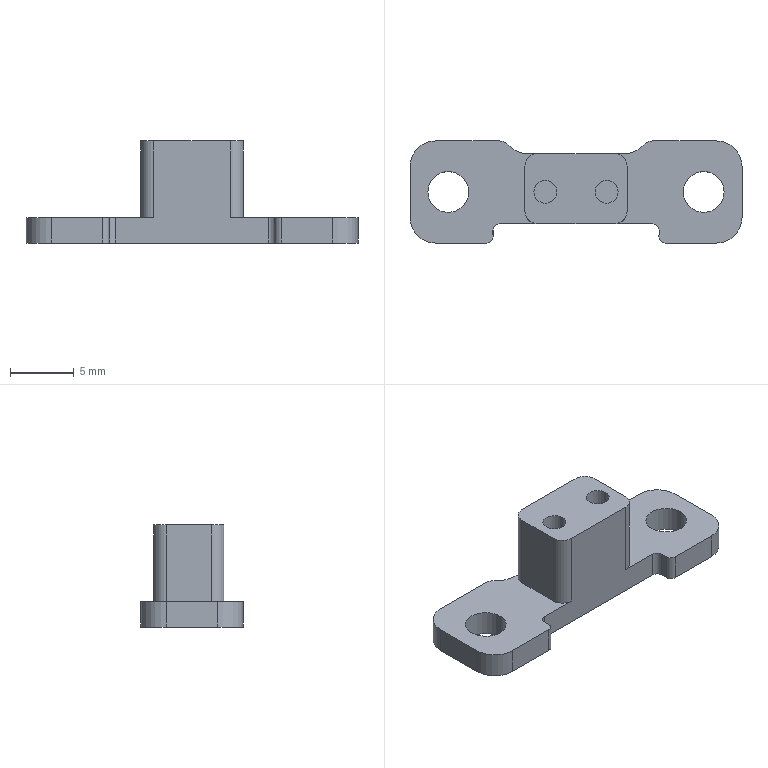CAM job | Mastercam | 3-axis milling, 5-axis milling, drilling | stock box 40 x 15 x 8 mm
Tools:
tool_number,name,type,diameter_mm,corner_radius_mm,flutes,flute_length_mm,overall_length_mm,shoulder_length_mm,holder_diameter_mm,length_offset,diameter_offset,default_rpm,default_feed_mm_min,default_plunge_mm_min,coolant
1,1 Flat End Mill,end mill,1,0,4,6,75,6,50,1,1,10000,1200,600,COOL_OFF
4,4 Flat End Mill,end mill,4,0,4,25,75,25,50,4,4,2500,300,600,COOL_OFF
6,6 Flat End Mill,end mill,6,0,4,25,75,25,50,6,6,1667,200.04,600,COOL_OFF
7,4 Chamfer Mill,chamfer mill,4,0,4,25,75,30,50,7,7,6250,750,600,COOL_OFF
8,8 Flat End Mill,end mill,8,0,4,25,75,25,50,8,8,1250,150,600,COOL_OFF
24,100 Flat End Mill,end mill,100,0,4,100,200,120,50,24,24,12000,4000,600,COOL_OFF
Operations:
seq,operation,operation_type,tool_number,tool_name,tool_diameter_mm,spindle_rpm,feed_mm_min,plunge_mm_min,retract_mm_min,cycle_time_s,wcs,posted,nc_file
1,Facing - [WCS: Plane] - [Tplane: Plane],Facing,24,100 Flat End Mill,100,4000,1000,600,1200,12.67,Plane,yes,.nc
2,3D High Speed (Dynamic OptiRough) - [WCS: Plane] - [Tplane: Plane],HighSpeed3D,8,8 Flat End Mill,8,7000,4000,600,1200,54.968,Plane,yes,.nc
3,Contour (2D) - [WCS: Plane] - [Tplane: Plane],Contour,8,8 Flat End Mill,8,8000,1000,600,1200,10.305,Plane,yes,.nc
4,Contour (2D) - [WCS: Plane] - [Tplane: Plane],Contour,8,8 Flat End Mill,8,8000,1000,600,1200,7.192,Plane,yes,.nc
5,Contour (Remachining) - [WCS: Plane] - [Tplane: Plane],Contour,4,4 Flat End Mill,4,6000,1000,600,1200,15.541,Plane,yes,.nc
6,Contour (Remachining) - [WCS: Plane] - [Tplane: Plane],Contour,1,1 Flat End Mill,1,6000,500,600,1200,20.97,Plane,yes,.nc
7,Drill/Counterbore - [WCS: Plane] - [Tplane: Plane],Drill,7,4 Chamfer Mill,4,6000,200,600,1200,4.02,Plane,yes,.nc
8,Deburr 5-axis - [WCS: Plane] - [Tplane: Plane],459,7,4 Chamfer Mill,4,6000,1000,600,1200,10.025,Plane,yes,.nc
9,Facing - [WCS: Plane-1] - [Tplane: Plane-1],Facing,6,6 Flat End Mill,6,8000,2000,600,1200,169.574,Plane-1,yes,.nc